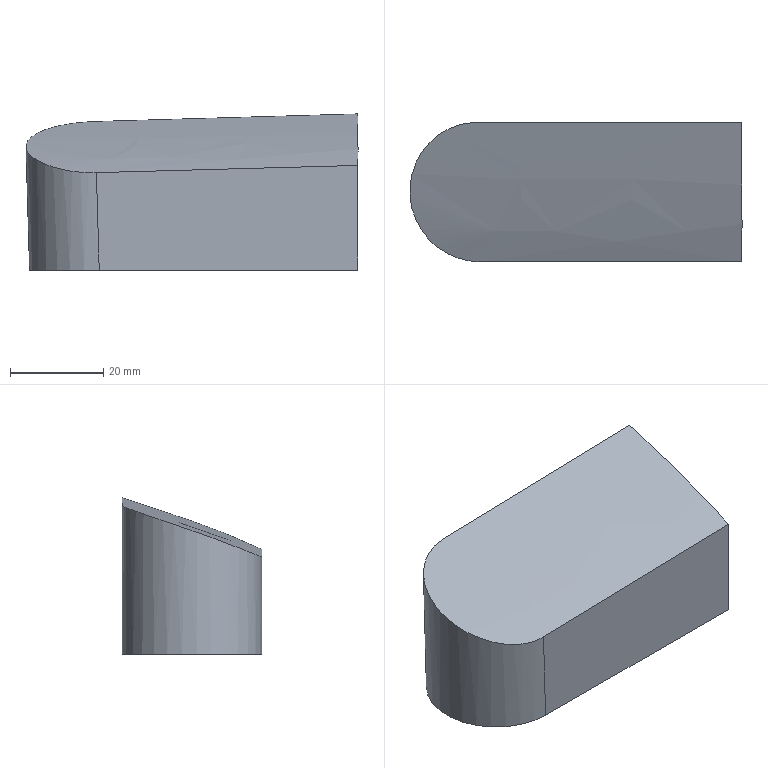Part | NX | features solid 2 | 1 solid | 6 faces | box 71.388 x 30 x 33.552 mm | volume 55801 mm3 | plane 4 | spline 1 | cylinder 1 | commonest cylinder face diameters 30 x1
STEP:
#1=CARTESIAN_POINT('',(-71.,-617.5,-10.));
#2=VERTEX_POINT('',#1);
#3=CARTESIAN_POINT('',(-71.,-647.5,-10.));
#4=VERTEX_POINT('',#3);
#5=CARTESIAN_POINT('',(-71.,-650.,-10.));
#6=DIRECTION('',(0.,1.,0.));
#7=VECTOR('',#6,1000.);
#8=LINE('',#5,#7);
#9=EDGE_CURVE('',#2,#4,#8,.F.);
#10=ORIENTED_EDGE('',*,*,#9,.F.);
#11=CARTESIAN_POINT('',(-71.,-617.5,23.552));
#12=VERTEX_POINT('',#11);
#13=CARTESIAN_POINT('',(-71.,-617.5,-115.));
#14=DIRECTION('',(0.,0.,1.));
#15=VECTOR('',#14,1000.);
#16=LINE('',#13,#15);
#17=EDGE_CURVE('',#12,#2,#16,.F.);
#18=ORIENTED_EDGE('',*,*,#17,.F.);
#19=CARTESIAN_POINT('',(-71.,-647.5,12.484));
#20=VERTEX_POINT('',#19);
#21=CARTESIAN_POINT('',(-71.,-617.5,23.552));
#22=CARTESIAN_POINT('',(-71.,-627.639,20.232));
#23=CARTESIAN_POINT('',(-71.,-637.892,17.101));
#24=CARTESIAN_POINT('',(-71.,-647.5,12.484));
#25=B_SPLINE_CURVE_WITH_KNOTS('',3,(#21,#22,#23,#24),.UNSPECIFIED.,.F.,.F.,(4,4),(0.1711,0.2032),.UNSPECIFIED.);
#26=EDGE_CURVE('',#12,#20,#25,.T.);
#27=ORIENTED_EDGE('',*,*,#26,.T.);
#28=CARTESIAN_POINT('',(-71.,-647.5,-115.));
#29=DIRECTION('',(0.,0.,1.));
#30=VECTOR('',#29,1000.);
#31=LINE('',#28,#30);
#32=EDGE_CURVE('',#20,#4,#31,.F.);
#33=ORIENTED_EDGE('',*,*,#32,.T.);
#34=EDGE_LOOP('',(#10,#18,#27,#33));
#35=FACE_BOUND('',#34,.T.);
#36=CARTESIAN_POINT('',(-71.,523.772,-115.));
#37=DIRECTION('',(1.,0.,0.));
#38=DIRECTION('',(0.,0.,-1.));
#39=AXIS2_PLACEMENT_3D('',#36,#37,#38);
#40=PLANE('',#39);
#41=ADVANCED_FACE('',(#35),#40,.T.);
#42=CARTESIAN_POINT('',(-127.217,-647.5,10.938));
#43=VERTEX_POINT('',#42);
#44=CARTESIAN_POINT('',(-127.217,-647.5,10.938));
#45=CARTESIAN_POINT('',(-108.479,-647.5,11.484));
#46=CARTESIAN_POINT('',(-89.739,-647.5,11.982));
#47=CARTESIAN_POINT('',(-71.,-647.5,12.484));
#48=B_SPLINE_CURVE_WITH_KNOTS('',3,(#44,#45,#46,#47),.UNSPECIFIED.,.F.,.F.,(4,4),(0.,0.05624),.UNSPECIFIED.);
#49=EDGE_CURVE('',#43,#20,#48,.T.);
#50=ORIENTED_EDGE('',*,*,#49,.F.);
#51=CARTESIAN_POINT('',(-126.603,-647.5,-10.));
#52=VERTEX_POINT('',#51);
#53=CARTESIAN_POINT('',(-126.616,-647.5,-9.56));
#54=DIRECTION('',(-0.02934,0.,0.9996));
#55=VECTOR('',#54,1000.);
#56=LINE('',#53,#55);
#57=EDGE_CURVE('',#43,#52,#56,.F.);
#58=ORIENTED_EDGE('',*,*,#57,.T.);
#59=CARTESIAN_POINT('',(10.,-647.5,-10.));
#60=DIRECTION('',(1.,0.,0.));
#61=VECTOR('',#60,1000.);
#62=LINE('',#59,#61);
#63=EDGE_CURVE('',#52,#4,#62,.T.);
#64=ORIENTED_EDGE('',*,*,#63,.T.);
#65=ORIENTED_EDGE('',*,*,#32,.F.);
#66=EDGE_LOOP('',(#50,#58,#64,#65));
#67=FACE_BOUND('',#66,.T.);
#68=CARTESIAN_POINT('',(10.,-647.5,5.));
#69=DIRECTION('',(0.,-1.,0.));
#70=DIRECTION('',(0.,0.,1.));
#71=AXIS2_PLACEMENT_3D('',#68,#69,#70);
#72=PLANE('',#71);
#73=ADVANCED_FACE('',(#67),#72,.T.);
#74=CARTESIAN_POINT('',(-126.603,-617.5,-10.));
#75=VERTEX_POINT('',#74);
#76=CARTESIAN_POINT('',(10.,-617.5,-10.));
#77=DIRECTION('',(-1.,0.,0.));
#78=VECTOR('',#77,1000.);
#79=LINE('',#76,#78);
#80=EDGE_CURVE('',#2,#75,#79,.T.);
#81=ORIENTED_EDGE('',*,*,#80,.T.);
#82=CARTESIAN_POINT('',(-127.54,-617.5,21.915));
#83=VERTEX_POINT('',#82);
#84=CARTESIAN_POINT('',(-127.693,-617.5,27.154));
#85=DIRECTION('',(0.02934,0.,-0.9996));
#86=VECTOR('',#85,1000.);
#87=LINE('',#84,#86);
#88=EDGE_CURVE('',#75,#83,#87,.F.);
#89=ORIENTED_EDGE('',*,*,#88,.T.);
#90=CARTESIAN_POINT('',(-71.,-617.5,23.552));
#91=CARTESIAN_POINT('',(-89.847,-617.5,23.015));
#92=CARTESIAN_POINT('',(-108.694,-617.5,22.482));
#93=CARTESIAN_POINT('',(-127.54,-617.5,21.915));
#94=B_SPLINE_CURVE_WITH_KNOTS('',3,(#90,#91,#92,#93),.UNSPECIFIED.,.F.,.F.,(4,4),(0.4078,0.4644),.UNSPECIFIED.);
#95=EDGE_CURVE('',#12,#83,#94,.T.);
#96=ORIENTED_EDGE('',*,*,#95,.F.);
#97=ORIENTED_EDGE('',*,*,#17,.T.);
#98=EDGE_LOOP('',(#81,#89,#96,#97));
#99=FACE_BOUND('',#98,.T.);
#100=CARTESIAN_POINT('',(10.,-617.5,5.));
#101=DIRECTION('',(0.,1.,0.));
#102=DIRECTION('',(0.,0.,-1.));
#103=AXIS2_PLACEMENT_3D('',#100,#101,#102);
#104=PLANE('',#103);
#105=ADVANCED_FACE('',(#99),#104,.T.);
#106=CARTESIAN_POINT('',(-127.54,-617.5,21.915));
#107=CARTESIAN_POINT('',(-129.56,-617.5,21.854));
#108=CARTESIAN_POINT('',(-133.61,-618.338,21.46));
#109=CARTESIAN_POINT('',(-140.268,-622.996,19.735));
#110=CARTESIAN_POINT('',(-143.91,-632.707,16.525));
#111=CARTESIAN_POINT('',(-139.931,-642.113,13.033));
#112=CARTESIAN_POINT('',(-133.294,-646.657,11.167));
#113=CARTESIAN_POINT('',(-129.241,-647.5,10.879));
#114=CARTESIAN_POINT('',(-127.217,-647.5,10.938));
#115=B_SPLINE_CURVE_WITH_KNOTS('',3,(#106,#107,#108,#109,#110,#111,#112,#113,#114),.UNSPECIFIED.,.F.,.F.,(4,1,1,1,1,1,4),(0.01344,0.01949,0.02554,0.03765,0.04976,0.05582,0.06187),.UNSPECIFIED.);
#116=EDGE_CURVE('',#83,#43,#115,.T.);
#117=ORIENTED_EDGE('',*,*,#116,.T.);
#118=ORIENTED_EDGE('',*,*,#49,.T.);
#119=ORIENTED_EDGE('',*,*,#26,.F.);
#120=ORIENTED_EDGE('',*,*,#95,.T.);
#121=EDGE_LOOP('',(#117,#118,#119,#120));
#122=FACE_BOUND('',#121,.T.);
#123=CARTESIAN_POINT('',(-70.068,-617.314,23.639));
#124=CARTESIAN_POINT('',(-94.508,-617.296,22.952));
#125=CARTESIAN_POINT('',(-118.931,-617.279,22.263));
#126=CARTESIAN_POINT('',(-143.361,-617.258,21.512));
#127=CARTESIAN_POINT('',(-70.109,-619.739,22.846));
#128=CARTESIAN_POINT('',(-94.512,-619.723,22.163));
#129=CARTESIAN_POINT('',(-118.899,-619.706,21.477));
#130=CARTESIAN_POINT('',(-143.293,-619.685,20.727));
#131=CARTESIAN_POINT('',(-70.164,-622.989,21.774));
#132=CARTESIAN_POINT('',(-94.519,-622.974,21.095));
#133=CARTESIAN_POINT('',(-118.856,-622.959,20.413));
#134=CARTESIAN_POINT('',(-143.2,-622.938,19.666));
#135=CARTESIAN_POINT('',(-70.235,-627.189,20.403));
#136=CARTESIAN_POINT('',(-94.527,-627.176,19.73));
#137=CARTESIAN_POINT('',(-118.801,-627.162,19.054));
#138=CARTESIAN_POINT('',(-143.082,-627.142,18.31));
#139=CARTESIAN_POINT('',(-70.291,-630.379,19.341));
#140=CARTESIAN_POINT('',(-94.534,-630.366,18.672));
#141=CARTESIAN_POINT('',(-118.758,-630.353,18.001));
#142=CARTESIAN_POINT('',(-142.989,-630.334,17.259));
#143=CARTESIAN_POINT('',(-70.41,-637.458,16.857));
#144=CARTESIAN_POINT('',(-94.545,-637.45,16.198));
#145=CARTESIAN_POINT('',(-118.659,-637.442,15.536));
#146=CARTESIAN_POINT('',(-142.782,-637.424,14.8));
#147=CARTESIAN_POINT('',(-70.509,-643.325,14.522));
#148=CARTESIAN_POINT('',(-94.549,-643.324,13.874));
#149=CARTESIAN_POINT('',(-118.568,-643.323,13.224));
#150=CARTESIAN_POINT('',(-142.596,-643.307,12.494));
#151=CARTESIAN_POINT('',(-70.577,-647.676,12.411));
#152=CARTESIAN_POINT('',(-94.544,-647.676,11.773));
#153=CARTESIAN_POINT('',(-118.49,-647.676,11.131));
#154=CARTESIAN_POINT('',(-142.444,-647.663,10.408));
#155=B_SPLINE_SURFACE_WITH_KNOTS('',3,3,((#123,#124,#125,#126),(#127,#128,#129,#130),(#131,#132,#133,#134),(#135,#136,#137,#138),(#139,#140,#141,#142),(#143,#144,#145,#146),(#147,#148,#149,#150),(#151,#152,#153,#154)),.UNSPECIFIED.,.F.,.F.,.F.,(4,1,1,1,1,4),(4,4),(-0.3421,-0.08979,0.001946,0.09368,0.2542,0.7588),(-0.04797,0.1009),.UNSPECIFIED.);
#156=ADVANCED_FACE('',(#122),#155,.F.);
#157=ORIENTED_EDGE('',*,*,#63,.F.);
#158=CARTESIAN_POINT('',(-126.603,-632.5,-10.));
#159=DIRECTION('',(0.,0.,-1.));
#160=DIRECTION('',(-1.,0.,0.));
#161=AXIS2_PLACEMENT_3D('',#158,#159,#160);
#162=ELLIPSE('',#161,15.006,15.);
#163=EDGE_CURVE('',#52,#75,#162,.T.);
#164=ORIENTED_EDGE('',*,*,#163,.T.);
#165=ORIENTED_EDGE('',*,*,#80,.F.);
#166=ORIENTED_EDGE('',*,*,#9,.T.);
#167=EDGE_LOOP('',(#157,#164,#165,#166));
#168=FACE_BOUND('',#167,.T.);
#169=CARTESIAN_POINT('',(10.,-650.,-10.));
#170=DIRECTION('',(0.,0.,-1.));
#171=DIRECTION('',(-1.,0.,0.));
#172=AXIS2_PLACEMENT_3D('',#169,#170,#171);
#173=PLANE('',#172);
#174=ADVANCED_FACE('',(#168),#173,.T.);
#175=ORIENTED_EDGE('',*,*,#88,.F.);
#176=ORIENTED_EDGE('',*,*,#163,.F.);
#177=ORIENTED_EDGE('',*,*,#57,.F.);
#178=ORIENTED_EDGE('',*,*,#116,.F.);
#179=EDGE_LOOP('',(#175,#176,#177,#178));
#180=FACE_BOUND('',#179,.T.);
#181=CARTESIAN_POINT('',(-127.498,-632.5,20.492));
#182=DIRECTION('',(-0.02934,0.,0.9996));
#183=DIRECTION('',(0.9996,0.,0.02934));
#184=AXIS2_PLACEMENT_3D('',#181,#182,#183);
#185=CYLINDRICAL_SURFACE('',#184,15.);
#186=ADVANCED_FACE('',(#180),#185,.T.);
#187=CLOSED_SHELL('',(#41,#73,#105,#156,#174,#186));
#188=MANIFOLD_SOLID_BREP('',#187);
#189=(LENGTH_UNIT()NAMED_UNIT(*)SI_UNIT(.MILLI.,.METRE.));
#190=UNCERTAINTY_MEASURE_WITH_UNIT(LENGTH_MEASURE(0.0508),#189,'','');
#191=(NAMED_UNIT(*)PLANE_ANGLE_UNIT()SI_UNIT($,.RADIAN.));
#192=(NAMED_UNIT(*)SI_UNIT($,.STERADIAN.)SOLID_ANGLE_UNIT());
#193=(GEOMETRIC_REPRESENTATION_CONTEXT(3)GLOBAL_UNCERTAINTY_ASSIGNED_CONTEXT((#190))GLOBAL_UNIT_ASSIGNED_CONTEXT((#189,#191,#192))REPRESENTATION_CONTEXT('',''));
#194=ADVANCED_BREP_SHAPE_REPRESENTATION('',(#188),#193);